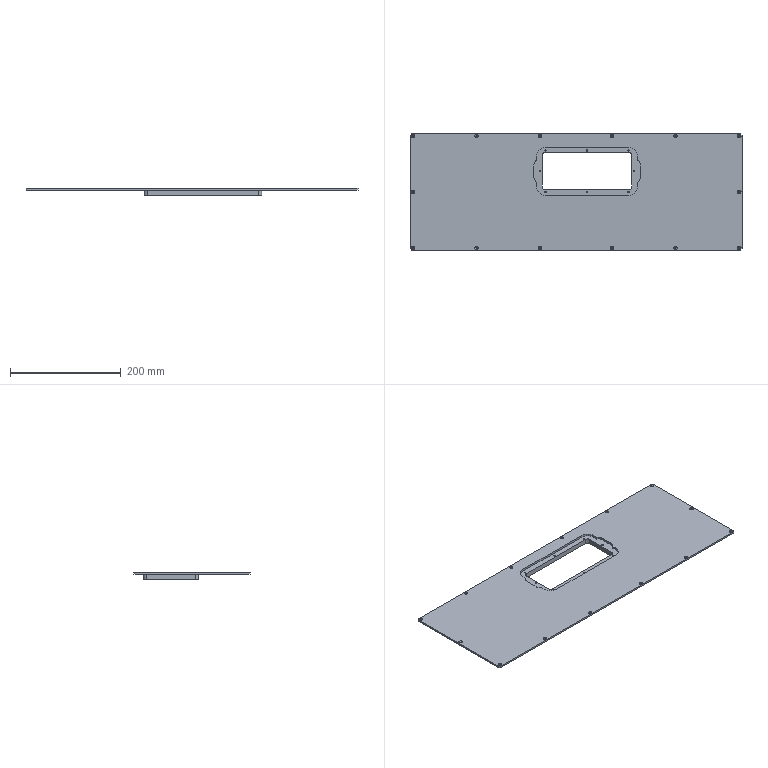Part | SolidWorks | features ICE 7, Fillet 4, Chamfer 2, 3DProfileFeature 1, Extrusion 1, HoleWzd 1 | 1 solid | 132 faces | box 600 x 210 x 13 mm | volume 425401 mm3 | cylinder 60 | cone 44 | plane 28 | commonest cylinder face diameters 3.5 x28 2.5 x16 10 x8 20 x4 32 x4